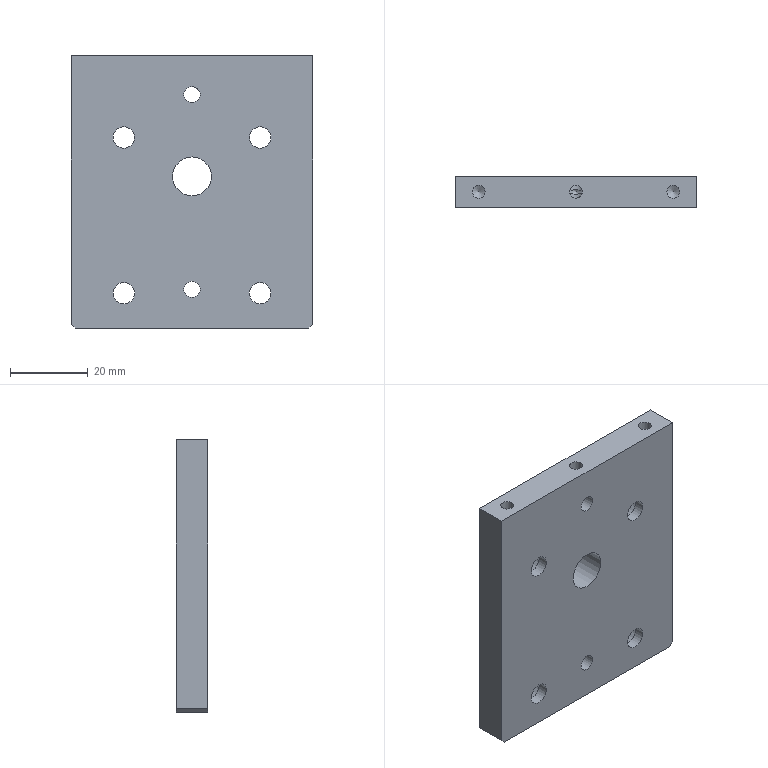Part | NX | 1 solid | 31 faces | box 62 x 8 x 70 mm | volume 31647 mm3 | cylinder 16 | plane 12 | cone 3 | commonest cylinder face diameters 3.3 x5 10 x5 5.5 x4 4.2 x2
STEP:
#1=CARTESIAN_POINT('',(-31.,4.,-34.));
#2=VERTEX_POINT('',#1);
#3=CARTESIAN_POINT('',(-31.,4.,35.));
#4=VERTEX_POINT('',#3);
#5=CARTESIAN_POINT('',(-31.,4.,35.));
#6=DIRECTION('',(0.,0.,1.));
#7=VECTOR('',#6,1000.);
#8=LINE('',#5,#7);
#9=EDGE_CURVE('',#2,#4,#8,.T.);
#10=ORIENTED_EDGE('',*,*,#9,.F.);
#11=CARTESIAN_POINT('',(-31.,-4.,-34.));
#12=VERTEX_POINT('',#11);
#13=CARTESIAN_POINT('',(-31.,4.,-34.));
#14=DIRECTION('',(0.,-1.,0.));
#15=VECTOR('',#14,1000.);
#16=LINE('',#13,#15);
#17=EDGE_CURVE('',#2,#12,#16,.T.);
#18=ORIENTED_EDGE('',*,*,#17,.T.);
#19=CARTESIAN_POINT('',(-31.,-4.,35.));
#20=VERTEX_POINT('',#19);
#21=CARTESIAN_POINT('',(-31.,-4.,35.));
#22=DIRECTION('',(0.,0.,1.));
#23=VECTOR('',#22,1000.);
#24=LINE('',#21,#23);
#25=EDGE_CURVE('',#12,#20,#24,.T.);
#26=ORIENTED_EDGE('',*,*,#25,.T.);
#27=CARTESIAN_POINT('',(-31.,4.,35.));
#28=DIRECTION('',(0.,-1.,0.));
#29=VECTOR('',#28,1000.);
#30=LINE('',#27,#29);
#31=EDGE_CURVE('',#4,#20,#30,.T.);
#32=ORIENTED_EDGE('',*,*,#31,.F.);
#33=EDGE_LOOP('',(#10,#18,#26,#32));
#34=FACE_BOUND('',#33,.T.);
#35=CARTESIAN_POINT('',(-31.,4.,35.));
#36=DIRECTION('',(1.,0.,0.));
#37=DIRECTION('',(0.,0.,-1.));
#38=AXIS2_PLACEMENT_3D('',#35,#36,#37);
#39=PLANE('',#38);
#40=ADVANCED_FACE('',(#34),#39,.F.);
#41=CARTESIAN_POINT('',(-23.35,0.,35.));
#42=VERTEX_POINT('',#41);
#43=CARTESIAN_POINT('',(-25.,0.,35.));
#44=DIRECTION('',(0.,0.,1.));
#45=DIRECTION('',(1.,0.,0.));
#46=AXIS2_PLACEMENT_3D('',#43,#44,#45);
#47=CIRCLE('',#46,1.65);
#48=EDGE_CURVE('',#42,#42,#47,.T.);
#49=ORIENTED_EDGE('',*,*,#48,.F.);
#50=EDGE_LOOP('',(#49));
#51=FACE_BOUND('',#50,.T.);
#52=CARTESIAN_POINT('',(1.65,0.,35.));
#53=VERTEX_POINT('',#52);
#54=CARTESIAN_POINT('',(0.,0.,35.));
#55=DIRECTION('',(0.,0.,1.));
#56=DIRECTION('',(1.,0.,0.));
#57=AXIS2_PLACEMENT_3D('',#54,#55,#56);
#58=CIRCLE('',#57,1.65);
#59=EDGE_CURVE('',#53,#53,#58,.T.);
#60=ORIENTED_EDGE('',*,*,#59,.F.);
#61=EDGE_LOOP('',(#60));
#62=FACE_BOUND('',#61,.T.);
#63=CARTESIAN_POINT('',(26.65,0.,35.));
#64=VERTEX_POINT('',#63);
#65=CARTESIAN_POINT('',(25.,0.,35.));
#66=DIRECTION('',(0.,0.,1.));
#67=DIRECTION('',(1.,0.,0.));
#68=AXIS2_PLACEMENT_3D('',#65,#66,#67);
#69=CIRCLE('',#68,1.65);
#70=EDGE_CURVE('',#64,#64,#69,.T.);
#71=ORIENTED_EDGE('',*,*,#70,.F.);
#72=EDGE_LOOP('',(#71));
#73=FACE_BOUND('',#72,.T.);
#74=CARTESIAN_POINT('',(31.,-4.,35.));
#75=VERTEX_POINT('',#74);
#76=CARTESIAN_POINT('',(31.,-4.,35.));
#77=DIRECTION('',(1.,0.,0.));
#78=VECTOR('',#77,1000.);
#79=LINE('',#76,#78);
#80=EDGE_CURVE('',#20,#75,#79,.T.);
#81=ORIENTED_EDGE('',*,*,#80,.T.);
#82=CARTESIAN_POINT('',(31.,4.,35.));
#83=VERTEX_POINT('',#82);
#84=CARTESIAN_POINT('',(31.,4.,35.));
#85=DIRECTION('',(0.,-1.,0.));
#86=VECTOR('',#85,1000.);
#87=LINE('',#84,#86);
#88=EDGE_CURVE('',#83,#75,#87,.T.);
#89=ORIENTED_EDGE('',*,*,#88,.F.);
#90=CARTESIAN_POINT('',(31.,4.,35.));
#91=DIRECTION('',(1.,0.,0.));
#92=VECTOR('',#91,1000.);
#93=LINE('',#90,#92);
#94=EDGE_CURVE('',#4,#83,#93,.T.);
#95=ORIENTED_EDGE('',*,*,#94,.F.);
#96=ORIENTED_EDGE('',*,*,#31,.T.);
#97=EDGE_LOOP('',(#81,#89,#95,#96));
#98=FACE_BOUND('',#97,.T.);
#99=CARTESIAN_POINT('',(31.,4.,35.));
#100=DIRECTION('',(0.,0.,-1.));
#101=DIRECTION('',(-1.,0.,0.));
#102=AXIS2_PLACEMENT_3D('',#99,#100,#101);
#103=PLANE('',#102);
#104=ADVANCED_FACE('',(#51,#62,#73,#98),#103,.F.);
#105=CARTESIAN_POINT('',(31.,-4.,-34.));
#106=VERTEX_POINT('',#105);
#107=CARTESIAN_POINT('',(31.,-4.,35.));
#108=DIRECTION('',(0.,0.,-1.));
#109=VECTOR('',#108,1000.);
#110=LINE('',#107,#109);
#111=EDGE_CURVE('',#75,#106,#110,.T.);
#112=ORIENTED_EDGE('',*,*,#111,.T.);
#113=CARTESIAN_POINT('',(31.,4.,-34.));
#114=VERTEX_POINT('',#113);
#115=CARTESIAN_POINT('',(31.,4.,-34.));
#116=DIRECTION('',(0.,1.,0.));
#117=VECTOR('',#116,1000.);
#118=LINE('',#115,#117);
#119=EDGE_CURVE('',#106,#114,#118,.T.);
#120=ORIENTED_EDGE('',*,*,#119,.T.);
#121=CARTESIAN_POINT('',(31.,4.,35.));
#122=DIRECTION('',(0.,0.,-1.));
#123=VECTOR('',#122,1000.);
#124=LINE('',#121,#123);
#125=EDGE_CURVE('',#83,#114,#124,.T.);
#126=ORIENTED_EDGE('',*,*,#125,.F.);
#127=ORIENTED_EDGE('',*,*,#88,.T.);
#128=EDGE_LOOP('',(#112,#120,#126,#127));
#129=FACE_BOUND('',#128,.T.);
#130=CARTESIAN_POINT('',(31.,4.,35.));
#131=DIRECTION('',(-1.,0.,0.));
#132=DIRECTION('',(0.,0.,1.));
#133=AXIS2_PLACEMENT_3D('',#130,#131,#132);
#134=PLANE('',#133);
#135=ADVANCED_FACE('',(#129),#134,.F.);
#136=CARTESIAN_POINT('',(30.,4.,-35.));
#137=VERTEX_POINT('',#136);
#138=CARTESIAN_POINT('',(-30.,4.,-35.));
#139=VERTEX_POINT('',#138);
#140=CARTESIAN_POINT('',(31.,4.,-35.));
#141=DIRECTION('',(-1.,0.,0.));
#142=VECTOR('',#141,1000.);
#143=LINE('',#140,#142);
#144=EDGE_CURVE('',#137,#139,#143,.T.);
#145=ORIENTED_EDGE('',*,*,#144,.F.);
#146=CARTESIAN_POINT('',(30.,-4.,-35.));
#147=VERTEX_POINT('',#146);
#148=CARTESIAN_POINT('',(30.,4.,-35.));
#149=DIRECTION('',(0.,-1.,0.));
#150=VECTOR('',#149,1000.);
#151=LINE('',#148,#150);
#152=EDGE_CURVE('',#137,#147,#151,.T.);
#153=ORIENTED_EDGE('',*,*,#152,.T.);
#154=CARTESIAN_POINT('',(-30.,-4.,-35.));
#155=VERTEX_POINT('',#154);
#156=CARTESIAN_POINT('',(31.,-4.,-35.));
#157=DIRECTION('',(-1.,0.,0.));
#158=VECTOR('',#157,1000.);
#159=LINE('',#156,#158);
#160=EDGE_CURVE('',#147,#155,#159,.T.);
#161=ORIENTED_EDGE('',*,*,#160,.T.);
#162=CARTESIAN_POINT('',(-30.,4.,-35.));
#163=DIRECTION('',(0.,1.,0.));
#164=VECTOR('',#163,1000.);
#165=LINE('',#162,#164);
#166=EDGE_CURVE('',#155,#139,#165,.T.);
#167=ORIENTED_EDGE('',*,*,#166,.T.);
#168=EDGE_LOOP('',(#145,#153,#161,#167));
#169=FACE_BOUND('',#168,.T.);
#170=CARTESIAN_POINT('',(31.,4.,-35.));
#171=DIRECTION('',(0.,0.,1.));
#172=DIRECTION('',(1.,0.,0.));
#173=AXIS2_PLACEMENT_3D('',#170,#171,#172);
#174=PLANE('',#173);
#175=ADVANCED_FACE('',(#169),#174,.F.);
#176=CARTESIAN_POINT('',(0.,4.,-22.9));
#177=VERTEX_POINT('',#176);
#178=CARTESIAN_POINT('',(0.,4.,-25.));
#179=DIRECTION('',(0.,1.,0.));
#180=DIRECTION('',(0.,0.,1.));
#181=AXIS2_PLACEMENT_3D('',#178,#179,#180);
#182=CIRCLE('',#181,2.1);
#183=EDGE_CURVE('',#177,#177,#182,.T.);
#184=ORIENTED_EDGE('',*,*,#183,.F.);
#185=EDGE_LOOP('',(#184));
#186=FACE_BOUND('',#185,.T.);
#187=CARTESIAN_POINT('',(0.,4.,27.1));
#188=VERTEX_POINT('',#187);
#189=CARTESIAN_POINT('',(0.,4.,25.));
#190=DIRECTION('',(0.,1.,0.));
#191=DIRECTION('',(0.,0.,1.));
#192=AXIS2_PLACEMENT_3D('',#189,#190,#191);
#193=CIRCLE('',#192,2.1);
#194=EDGE_CURVE('',#188,#188,#193,.T.);
#195=ORIENTED_EDGE('',*,*,#194,.F.);
#196=EDGE_LOOP('',(#195));
#197=FACE_BOUND('',#196,.T.);
#198=CARTESIAN_POINT('',(0.,4.,9.));
#199=VERTEX_POINT('',#198);
#200=CARTESIAN_POINT('',(0.,4.,4.));
#201=DIRECTION('',(0.,1.,0.));
#202=DIRECTION('',(0.,0.,1.));
#203=AXIS2_PLACEMENT_3D('',#200,#201,#202);
#204=CIRCLE('',#203,5.);
#205=EDGE_CURVE('',#199,#199,#204,.T.);
#206=ORIENTED_EDGE('',*,*,#205,.F.);
#207=EDGE_LOOP('',(#206));
#208=FACE_BOUND('',#207,.T.);
#209=CARTESIAN_POINT('',(-17.5,4.,-21.));
#210=VERTEX_POINT('',#209);
#211=CARTESIAN_POINT('',(-17.5,4.,-26.));
#212=DIRECTION('',(0.,1.,0.));
#213=DIRECTION('',(0.,0.,1.));
#214=AXIS2_PLACEMENT_3D('',#211,#212,#213);
#215=CIRCLE('',#214,5.);
#216=EDGE_CURVE('',#210,#210,#215,.T.);
#217=ORIENTED_EDGE('',*,*,#216,.F.);
#218=EDGE_LOOP('',(#217));
#219=FACE_BOUND('',#218,.T.);
#220=CARTESIAN_POINT('',(17.5,4.,-21.));
#221=VERTEX_POINT('',#220);
#222=CARTESIAN_POINT('',(17.5,4.,-26.));
#223=DIRECTION('',(0.,1.,0.));
#224=DIRECTION('',(0.,0.,1.));
#225=AXIS2_PLACEMENT_3D('',#222,#223,#224);
#226=CIRCLE('',#225,5.);
#227=EDGE_CURVE('',#221,#221,#226,.T.);
#228=ORIENTED_EDGE('',*,*,#227,.F.);
#229=EDGE_LOOP('',(#228));
#230=FACE_BOUND('',#229,.T.);
#231=CARTESIAN_POINT('',(-17.5,4.,19.));
#232=VERTEX_POINT('',#231);
#233=CARTESIAN_POINT('',(-17.5,4.,14.));
#234=DIRECTION('',(0.,1.,0.));
#235=DIRECTION('',(0.,0.,1.));
#236=AXIS2_PLACEMENT_3D('',#233,#234,#235);
#237=CIRCLE('',#236,5.);
#238=EDGE_CURVE('',#232,#232,#237,.T.);
#239=ORIENTED_EDGE('',*,*,#238,.F.);
#240=EDGE_LOOP('',(#239));
#241=FACE_BOUND('',#240,.T.);
#242=CARTESIAN_POINT('',(17.5,4.,19.));
#243=VERTEX_POINT('',#242);
#244=CARTESIAN_POINT('',(17.5,4.,14.));
#245=DIRECTION('',(0.,1.,0.));
#246=DIRECTION('',(0.,0.,1.));
#247=AXIS2_PLACEMENT_3D('',#244,#245,#246);
#248=CIRCLE('',#247,5.);
#249=EDGE_CURVE('',#243,#243,#248,.T.);
#250=ORIENTED_EDGE('',*,*,#249,.F.);
#251=EDGE_LOOP('',(#250));
#252=FACE_BOUND('',#251,.T.);
#253=ORIENTED_EDGE('',*,*,#125,.T.);
#254=CARTESIAN_POINT('',(32.5,4.,-32.5));
#255=DIRECTION('',(0.7071,0.,0.7071));
#256=VECTOR('',#255,1000.);
#257=LINE('',#254,#256);
#258=EDGE_CURVE('',#114,#137,#257,.F.);
#259=ORIENTED_EDGE('',*,*,#258,.T.);
#260=ORIENTED_EDGE('',*,*,#144,.T.);
#261=CARTESIAN_POINT('',(-32.5,4.,-32.5));
#262=DIRECTION('',(0.7071,0.,-0.7071));
#263=VECTOR('',#262,1000.);
#264=LINE('',#261,#263);
#265=EDGE_CURVE('',#139,#2,#264,.F.);
#266=ORIENTED_EDGE('',*,*,#265,.T.);
#267=ORIENTED_EDGE('',*,*,#9,.T.);
#268=ORIENTED_EDGE('',*,*,#94,.T.);
#269=EDGE_LOOP('',(#253,#259,#260,#266,#267,#268));
#270=FACE_BOUND('',#269,.T.);
#271=CARTESIAN_POINT('',(0.,4.,0.));
#272=DIRECTION('',(0.,1.,0.));
#273=DIRECTION('',(0.,0.,1.));
#274=AXIS2_PLACEMENT_3D('',#271,#272,#273);
#275=PLANE('',#274);
#276=ADVANCED_FACE('',(#186,#197,#208,#219,#230,#241,#252,#270),#275,.T.);
#277=CARTESIAN_POINT('',(0.,-4.,-22.9));
#278=VERTEX_POINT('',#277);
#279=CARTESIAN_POINT('',(0.,-4.,-25.));
#280=DIRECTION('',(0.,1.,0.));
#281=DIRECTION('',(0.,0.,1.));
#282=AXIS2_PLACEMENT_3D('',#279,#280,#281);
#283=CIRCLE('',#282,2.1);
#284=EDGE_CURVE('',#278,#278,#283,.T.);
#285=ORIENTED_EDGE('',*,*,#284,.T.);
#286=EDGE_LOOP('',(#285));
#287=FACE_BOUND('',#286,.T.);
#288=CARTESIAN_POINT('',(0.,-4.,27.1));
#289=VERTEX_POINT('',#288);
#290=CARTESIAN_POINT('',(0.,-4.,25.));
#291=DIRECTION('',(0.,1.,0.));
#292=DIRECTION('',(0.,0.,1.));
#293=AXIS2_PLACEMENT_3D('',#290,#291,#292);
#294=CIRCLE('',#293,2.1);
#295=EDGE_CURVE('',#289,#289,#294,.T.);
#296=ORIENTED_EDGE('',*,*,#295,.T.);
#297=EDGE_LOOP('',(#296));
#298=FACE_BOUND('',#297,.T.);
#299=CARTESIAN_POINT('',(0.,-4.,9.));
#300=VERTEX_POINT('',#299);
#301=CARTESIAN_POINT('',(0.,-4.,4.));
#302=DIRECTION('',(0.,1.,0.));
#303=DIRECTION('',(0.,0.,1.));
#304=AXIS2_PLACEMENT_3D('',#301,#302,#303);
#305=CIRCLE('',#304,5.);
#306=EDGE_CURVE('',#300,#300,#305,.T.);
#307=ORIENTED_EDGE('',*,*,#306,.T.);
#308=EDGE_LOOP('',(#307));
#309=FACE_BOUND('',#308,.T.);
#310=CARTESIAN_POINT('',(-17.5,-4.,-23.25));
#311=VERTEX_POINT('',#310);
#312=CARTESIAN_POINT('',(-17.5,-4.,-26.));
#313=DIRECTION('',(0.,1.,0.));
#314=DIRECTION('',(0.,0.,1.));
#315=AXIS2_PLACEMENT_3D('',#312,#313,#314);
#316=CIRCLE('',#315,2.75);
#317=EDGE_CURVE('',#311,#311,#316,.T.);
#318=ORIENTED_EDGE('',*,*,#317,.T.);
#319=EDGE_LOOP('',(#318));
#320=FACE_BOUND('',#319,.T.);
#321=CARTESIAN_POINT('',(17.5,-4.,-23.25));
#322=VERTEX_POINT('',#321);
#323=CARTESIAN_POINT('',(17.5,-4.,-26.));
#324=DIRECTION('',(0.,1.,0.));
#325=DIRECTION('',(0.,0.,1.));
#326=AXIS2_PLACEMENT_3D('',#323,#324,#325);
#327=CIRCLE('',#326,2.75);
#328=EDGE_CURVE('',#322,#322,#327,.T.);
#329=ORIENTED_EDGE('',*,*,#328,.T.);
#330=EDGE_LOOP('',(#329));
#331=FACE_BOUND('',#330,.T.);
#332=CARTESIAN_POINT('',(-17.5,-4.,16.75));
#333=VERTEX_POINT('',#332);
#334=CARTESIAN_POINT('',(-17.5,-4.,14.));
#335=DIRECTION('',(0.,1.,0.));
#336=DIRECTION('',(0.,0.,1.));
#337=AXIS2_PLACEMENT_3D('',#334,#335,#336);
#338=CIRCLE('',#337,2.75);
#339=EDGE_CURVE('',#333,#333,#338,.T.);
#340=ORIENTED_EDGE('',*,*,#339,.T.);
#341=EDGE_LOOP('',(#340));
#342=FACE_BOUND('',#341,.T.);
#343=CARTESIAN_POINT('',(17.5,-4.,16.75));
#344=VERTEX_POINT('',#343);
#345=CARTESIAN_POINT('',(17.5,-4.,14.));
#346=DIRECTION('',(0.,1.,0.));
#347=DIRECTION('',(0.,0.,1.));
#348=AXIS2_PLACEMENT_3D('',#345,#346,#347);
#349=CIRCLE('',#348,2.75);
#350=EDGE_CURVE('',#344,#344,#349,.T.);
#351=ORIENTED_EDGE('',*,*,#350,.T.);
#352=EDGE_LOOP('',(#351));
#353=FACE_BOUND('',#352,.T.);
#354=ORIENTED_EDGE('',*,*,#160,.F.);
#355=CARTESIAN_POINT('',(30.,-4.,-35.));
#356=DIRECTION('',(-0.7071,0.,-0.7071));
#357=VECTOR('',#356,1000.);
#358=LINE('',#355,#357);
#359=EDGE_CURVE('',#147,#106,#358,.F.);
#360=ORIENTED_EDGE('',*,*,#359,.T.);
#361=ORIENTED_EDGE('',*,*,#111,.F.);
#362=ORIENTED_EDGE('',*,*,#80,.F.);
#363=ORIENTED_EDGE('',*,*,#25,.F.);
#364=CARTESIAN_POINT('',(-31.,-4.,-34.));
#365=DIRECTION('',(-0.7071,0.,0.7071));
#366=VECTOR('',#365,1000.);
#367=LINE('',#364,#366);
#368=EDGE_CURVE('',#12,#155,#367,.F.);
#369=ORIENTED_EDGE('',*,*,#368,.T.);
#370=EDGE_LOOP('',(#354,#360,#361,#362,#363,#369));
#371=FACE_BOUND('',#370,.T.);
#372=CARTESIAN_POINT('',(0.,-4.,0.));
#373=DIRECTION('',(0.,1.,0.));
#374=DIRECTION('',(0.,0.,1.));
#375=AXIS2_PLACEMENT_3D('',#372,#373,#374);
#376=PLANE('',#375);
#377=ADVANCED_FACE('',(#287,#298,#309,#320,#331,#342,#353,#371),#376,.F.);
#378=ORIENTED_EDGE('',*,*,#350,.F.);
#379=EDGE_LOOP('',(#378));
#380=FACE_BOUND('',#379,.T.);
#381=CARTESIAN_POINT('',(17.5,-1.4,16.75));
#382=VERTEX_POINT('',#381);
#383=CARTESIAN_POINT('',(17.5,-1.4,14.));
#384=DIRECTION('',(0.,1.,0.));
#385=DIRECTION('',(0.,0.,1.));
#386=AXIS2_PLACEMENT_3D('',#383,#384,#385);
#387=CIRCLE('',#386,2.75);
#388=EDGE_CURVE('',#382,#382,#387,.T.);
#389=ORIENTED_EDGE('',*,*,#388,.T.);
#390=EDGE_LOOP('',(#389));
#391=FACE_BOUND('',#390,.T.);
#392=CARTESIAN_POINT('',(17.5,4.,14.));
#393=DIRECTION('',(0.,1.,0.));
#394=DIRECTION('',(0.,0.,1.));
#395=AXIS2_PLACEMENT_3D('',#392,#393,#394);
#396=CYLINDRICAL_SURFACE('',#395,2.75);
#397=ADVANCED_FACE('',(#380,#391),#396,.F.);
#398=ORIENTED_EDGE('',*,*,#388,.F.);
#399=EDGE_LOOP('',(#398));
#400=FACE_BOUND('',#399,.T.);
#401=CARTESIAN_POINT('',(17.5,-1.4,19.));
#402=VERTEX_POINT('',#401);
#403=CARTESIAN_POINT('',(17.5,-1.4,14.));
#404=DIRECTION('',(0.,1.,0.));
#405=DIRECTION('',(0.,0.,1.));
#406=AXIS2_PLACEMENT_3D('',#403,#404,#405);
#407=CIRCLE('',#406,5.);
#408=EDGE_CURVE('',#402,#402,#407,.T.);
#409=ORIENTED_EDGE('',*,*,#408,.T.);
#410=EDGE_LOOP('',(#409));
#411=FACE_BOUND('',#410,.T.);
#412=CARTESIAN_POINT('',(20.25,-1.4,14.));
#413=DIRECTION('',(0.,-1.,0.));
#414=DIRECTION('',(0.,0.,-1.));
#415=AXIS2_PLACEMENT_3D('',#412,#413,#414);
#416=PLANE('',#415);
#417=ADVANCED_FACE('',(#400,#411),#416,.F.);
#418=ORIENTED_EDGE('',*,*,#408,.F.);
#419=EDGE_LOOP('',(#418));
#420=FACE_BOUND('',#419,.T.);
#421=ORIENTED_EDGE('',*,*,#249,.T.);
#422=EDGE_LOOP('',(#421));
#423=FACE_BOUND('',#422,.T.);
#424=CARTESIAN_POINT('',(17.5,4.,14.));
#425=DIRECTION('',(0.,1.,0.));
#426=DIRECTION('',(0.,0.,1.));
#427=AXIS2_PLACEMENT_3D('',#424,#425,#426);
#428=CYLINDRICAL_SURFACE('',#427,5.);
#429=ADVANCED_FACE('',(#420,#423),#428,.F.);
#430=ORIENTED_EDGE('',*,*,#339,.F.);
#431=EDGE_LOOP('',(#430));
#432=FACE_BOUND('',#431,.T.);
#433=CARTESIAN_POINT('',(-17.5,-1.4,16.75));
#434=VERTEX_POINT('',#433);
#435=CARTESIAN_POINT('',(-17.5,-1.4,14.));
#436=DIRECTION('',(0.,1.,0.));
#437=DIRECTION('',(0.,0.,1.));
#438=AXIS2_PLACEMENT_3D('',#435,#436,#437);
#439=CIRCLE('',#438,2.75);
#440=EDGE_CURVE('',#434,#434,#439,.T.);
#441=ORIENTED_EDGE('',*,*,#440,.T.);
#442=EDGE_LOOP('',(#441));
#443=FACE_BOUND('',#442,.T.);
#444=CARTESIAN_POINT('',(-17.5,4.,14.));
#445=DIRECTION('',(0.,1.,0.));
#446=DIRECTION('',(0.,0.,1.));
#447=AXIS2_PLACEMENT_3D('',#444,#445,#446);
#448=CYLINDRICAL_SURFACE('',#447,2.75);
#449=ADVANCED_FACE('',(#432,#443),#448,.F.);
#450=ORIENTED_EDGE('',*,*,#440,.F.);
#451=EDGE_LOOP('',(#450));
#452=FACE_BOUND('',#451,.T.);
#453=CARTESIAN_POINT('',(-17.5,-1.4,19.));
#454=VERTEX_POINT('',#453);
#455=CARTESIAN_POINT('',(-17.5,-1.4,14.));
#456=DIRECTION('',(0.,1.,0.));
#457=DIRECTION('',(0.,0.,1.));
#458=AXIS2_PLACEMENT_3D('',#455,#456,#457);
#459=CIRCLE('',#458,5.);
#460=EDGE_CURVE('',#454,#454,#459,.T.);
#461=ORIENTED_EDGE('',*,*,#460,.T.);
#462=EDGE_LOOP('',(#461));
#463=FACE_BOUND('',#462,.T.);
#464=CARTESIAN_POINT('',(-14.75,-1.4,14.));
#465=DIRECTION('',(0.,-1.,0.));
#466=DIRECTION('',(0.,0.,-1.));
#467=AXIS2_PLACEMENT_3D('',#464,#465,#466);
#468=PLANE('',#467);
#469=ADVANCED_FACE('',(#452,#463),#468,.F.);
#470=ORIENTED_EDGE('',*,*,#460,.F.);
#471=EDGE_LOOP('',(#470));
#472=FACE_BOUND('',#471,.T.);
#473=ORIENTED_EDGE('',*,*,#238,.T.);
#474=EDGE_LOOP('',(#473));
#475=FACE_BOUND('',#474,.T.);
#476=CARTESIAN_POINT('',(-17.5,4.,14.));
#477=DIRECTION('',(0.,1.,0.));
#478=DIRECTION('',(0.,0.,1.));
#479=AXIS2_PLACEMENT_3D('',#476,#477,#478);
#480=CYLINDRICAL_SURFACE('',#479,5.);
#481=ADVANCED_FACE('',(#472,#475),#480,.F.);
#482=ORIENTED_EDGE('',*,*,#328,.F.);
#483=EDGE_LOOP('',(#482));
#484=FACE_BOUND('',#483,.T.);
#485=CARTESIAN_POINT('',(17.5,-1.4,-23.25));
#486=VERTEX_POINT('',#485);
#487=CARTESIAN_POINT('',(17.5,-1.4,-26.));
#488=DIRECTION('',(0.,1.,0.));
#489=DIRECTION('',(0.,0.,1.));
#490=AXIS2_PLACEMENT_3D('',#487,#488,#489);
#491=CIRCLE('',#490,2.75);
#492=EDGE_CURVE('',#486,#486,#491,.T.);
#493=ORIENTED_EDGE('',*,*,#492,.T.);
#494=EDGE_LOOP('',(#493));
#495=FACE_BOUND('',#494,.T.);
#496=CARTESIAN_POINT('',(17.5,4.,-26.));
#497=DIRECTION('',(0.,1.,0.));
#498=DIRECTION('',(0.,0.,1.));
#499=AXIS2_PLACEMENT_3D('',#496,#497,#498);
#500=CYLINDRICAL_SURFACE('',#499,2.75);
#501=ADVANCED_FACE('',(#484,#495),#500,.F.);
#502=ORIENTED_EDGE('',*,*,#492,.F.);
#503=EDGE_LOOP('',(#502));
#504=FACE_BOUND('',#503,.T.);
#505=CARTESIAN_POINT('',(17.5,-1.4,-21.));
#506=VERTEX_POINT('',#505);
#507=CARTESIAN_POINT('',(17.5,-1.4,-26.));
#508=DIRECTION('',(0.,1.,0.));
#509=DIRECTION('',(0.,0.,1.));
#510=AXIS2_PLACEMENT_3D('',#507,#508,#509);
#511=CIRCLE('',#510,5.);
#512=EDGE_CURVE('',#506,#506,#511,.T.);
#513=ORIENTED_EDGE('',*,*,#512,.T.);
#514=EDGE_LOOP('',(#513));
#515=FACE_BOUND('',#514,.T.);
#516=CARTESIAN_POINT('',(20.25,-1.4,-26.));
#517=DIRECTION('',(0.,-1.,0.));
#518=DIRECTION('',(0.,0.,-1.));
#519=AXIS2_PLACEMENT_3D('',#516,#517,#518);
#520=PLANE('',#519);
#521=ADVANCED_FACE('',(#504,#515),#520,.F.);
#522=ORIENTED_EDGE('',*,*,#512,.F.);
#523=EDGE_LOOP('',(#522));
#524=FACE_BOUND('',#523,.T.);
#525=ORIENTED_EDGE('',*,*,#227,.T.);
#526=EDGE_LOOP('',(#525));
#527=FACE_BOUND('',#526,.T.);
#528=CARTESIAN_POINT('',(17.5,4.,-26.));
#529=DIRECTION('',(0.,1.,0.));
#530=DIRECTION('',(0.,0.,1.));
#531=AXIS2_PLACEMENT_3D('',#528,#529,#530);
#532=CYLINDRICAL_SURFACE('',#531,5.);
#533=ADVANCED_FACE('',(#524,#527),#532,.F.);
#534=ORIENTED_EDGE('',*,*,#317,.F.);
#535=EDGE_LOOP('',(#534));
#536=FACE_BOUND('',#535,.T.);
#537=CARTESIAN_POINT('',(-17.5,-1.4,-23.25));
#538=VERTEX_POINT('',#537);
#539=CARTESIAN_POINT('',(-17.5,-1.4,-26.));
#540=DIRECTION('',(0.,1.,0.));
#541=DIRECTION('',(0.,0.,1.));
#542=AXIS2_PLACEMENT_3D('',#539,#540,#541);
#543=CIRCLE('',#542,2.75);
#544=EDGE_CURVE('',#538,#538,#543,.T.);
#545=ORIENTED_EDGE('',*,*,#544,.T.);
#546=EDGE_LOOP('',(#545));
#547=FACE_BOUND('',#546,.T.);
#548=CARTESIAN_POINT('',(-17.5,4.,-26.));
#549=DIRECTION('',(0.,1.,0.));
#550=DIRECTION('',(0.,0.,1.));
#551=AXIS2_PLACEMENT_3D('',#548,#549,#550);
#552=CYLINDRICAL_SURFACE('',#551,2.75);
#553=ADVANCED_FACE('',(#536,#547),#552,.F.);
#554=ORIENTED_EDGE('',*,*,#544,.F.);
#555=EDGE_LOOP('',(#554));
#556=FACE_BOUND('',#555,.T.);
#557=CARTESIAN_POINT('',(-17.5,-1.4,-21.));
#558=VERTEX_POINT('',#557);
#559=CARTESIAN_POINT('',(-17.5,-1.4,-26.));
#560=DIRECTION('',(0.,1.,0.));
#561=DIRECTION('',(0.,0.,1.));
#562=AXIS2_PLACEMENT_3D('',#559,#560,#561);
#563=CIRCLE('',#562,5.);
#564=EDGE_CURVE('',#558,#558,#563,.T.);
#565=ORIENTED_EDGE('',*,*,#564,.T.);
#566=EDGE_LOOP('',(#565));
#567=FACE_BOUND('',#566,.T.);
#568=CARTESIAN_POINT('',(-14.75,-1.4,-26.));
#569=DIRECTION('',(0.,-1.,0.));
#570=DIRECTION('',(0.,0.,-1.));
#571=AXIS2_PLACEMENT_3D('',#568,#569,#570);
#572=PLANE('',#571);
#573=ADVANCED_FACE('',(#556,#567),#572,.F.);
#574=ORIENTED_EDGE('',*,*,#564,.F.);
#575=EDGE_LOOP('',(#574));
#576=FACE_BOUND('',#575,.T.);
#577=ORIENTED_EDGE('',*,*,#216,.T.);
#578=EDGE_LOOP('',(#577));
#579=FACE_BOUND('',#578,.T.);
#580=CARTESIAN_POINT('',(-17.5,4.,-26.));
#581=DIRECTION('',(0.,1.,0.));
#582=DIRECTION('',(0.,0.,1.));
#583=AXIS2_PLACEMENT_3D('',#580,#581,#582);
#584=CYLINDRICAL_SURFACE('',#583,5.);
#585=ADVANCED_FACE('',(#576,#579),#584,.F.);
#586=CARTESIAN_POINT('',(25.,0.,22.509));
#587=VERTEX_POINT('',#586);
#588=VERTEX_LOOP('',#587);
#589=FACE_BOUND('',#588,.T.);
#590=CARTESIAN_POINT('',(26.65,0.,23.5));
#591=VERTEX_POINT('',#590);
#592=CARTESIAN_POINT('',(25.,0.,23.5));
#593=DIRECTION('',(0.,0.,1.));
#594=DIRECTION('',(1.,0.,0.));
#595=AXIS2_PLACEMENT_3D('',#592,#593,#594);
#596=CIRCLE('',#595,1.65);
#597=EDGE_CURVE('',#591,#591,#596,.T.);
#598=ORIENTED_EDGE('',*,*,#597,.T.);
#599=EDGE_LOOP('',(#598));
#600=FACE_BOUND('',#599,.T.);
#601=CARTESIAN_POINT('',(25.,0.,23.5));
#602=DIRECTION('',(0.,0.,1.));
#603=DIRECTION('',(1.,0.,0.));
#604=AXIS2_PLACEMENT_3D('',#601,#602,#603);
#605=CONICAL_SURFACE('',#604,1.65,1.03);
#606=ADVANCED_FACE('',(#589,#600),#605,.F.);
#607=ORIENTED_EDGE('',*,*,#597,.F.);
#608=EDGE_LOOP('',(#607));
#609=FACE_BOUND('',#608,.T.);
#610=ORIENTED_EDGE('',*,*,#70,.T.);
#611=EDGE_LOOP('',(#610));
#612=FACE_BOUND('',#611,.T.);
#613=CARTESIAN_POINT('',(25.,0.,35.));
#614=DIRECTION('',(0.,0.,1.));
#615=DIRECTION('',(1.,0.,0.));
#616=AXIS2_PLACEMENT_3D('',#613,#614,#615);
#617=CYLINDRICAL_SURFACE('',#616,1.65);
#618=ADVANCED_FACE('',(#609,#612),#617,.F.);
#619=CARTESIAN_POINT('',(1.65,0.,26.299));
#620=VERTEX_POINT('',#619);
#621=CARTESIAN_POINT('',(1.55,0.6771,26.43));
#622=CARTESIAN_POINT('',(1.744,-0.2353,26.172));
#623=CARTESIAN_POINT('',(1.307,-1.268,26.781));
#624=CARTESIAN_POINT('',(0.004688,-1.838,27.259));
#625=CARTESIAN_POINT('',(-1.307,-1.279,26.782));
#626=CARTESIAN_POINT('',(-1.821,-0.0003141,26.059));
#627=CARTESIAN_POINT('',(-1.309,1.273,26.778));
#628=CARTESIAN_POINT('',(-0.007469,1.844,27.262));
#629=CARTESIAN_POINT('',(1.097,1.351,26.856));
#630=CARTESIAN_POINT('',(1.55,0.6771,26.43));
#631=CARTESIAN_POINT('',(1.744,-0.2353,26.172));
#632=CARTESIAN_POINT('',(1.307,-1.268,26.781));
#633=B_SPLINE_CURVE_WITH_KNOTS('',3,(#621,#622,#623,#624,#625,#626,#627,#628,#629,#630,#631,#632),.UNSPECIFIED.,.T.,.F.,(1,1,1,1,1,1,1,1,1,1,1,1,1,1,1,1),(-0.002727,-0.001364,-0.0006818,0.,0.001364,0.002727,0.004091,0.005454,0.006818,0.008181,0.009545,0.01023,0.01091,0.01227,0.01364,0.015),.UNSPECIFIED.);
#634=EDGE_CURVE('',#620,#620,#633,.T.);
#635=ORIENTED_EDGE('',*,*,#634,.T.);
#636=EDGE_LOOP('',(#635));
#637=FACE_BOUND('',#636,.T.);
#638=ORIENTED_EDGE('',*,*,#59,.T.);
#639=EDGE_LOOP('',(#638));
#640=FACE_BOUND('',#639,.T.);
#641=CARTESIAN_POINT('',(0.,0.,35.));
#642=DIRECTION('',(0.,0.,1.));
#643=DIRECTION('',(1.,0.,0.));
#644=AXIS2_PLACEMENT_3D('',#641,#642,#643);
#645=CYLINDRICAL_SURFACE('',#644,1.65);
#646=ADVANCED_FACE('',(#637,#640),#645,.F.);
#647=CARTESIAN_POINT('',(-25.,0.,22.509));
#648=VERTEX_POINT('',#647);
#649=VERTEX_LOOP('',#648);
#650=FACE_BOUND('',#649,.T.);
#651=CARTESIAN_POINT('',(-23.35,0.,23.5));
#652=VERTEX_POINT('',#651);
#653=CARTESIAN_POINT('',(-25.,0.,23.5));
#654=DIRECTION('',(0.,0.,1.));
#655=DIRECTION('',(1.,0.,0.));
#656=AXIS2_PLACEMENT_3D('',#653,#654,#655);
#657=CIRCLE('',#656,1.65);
#658=EDGE_CURVE('',#652,#652,#657,.T.);
#659=ORIENTED_EDGE('',*,*,#658,.T.);
#660=EDGE_LOOP('',(#659));
#661=FACE_BOUND('',#660,.T.);
#662=CARTESIAN_POINT('',(-25.,0.,23.5));
#663=DIRECTION('',(0.,0.,1.));
#664=DIRECTION('',(1.,0.,0.));
#665=AXIS2_PLACEMENT_3D('',#662,#663,#664);
#666=CONICAL_SURFACE('',#665,1.65,1.03);
#667=ADVANCED_FACE('',(#650,#661),#666,.F.);
#668=ORIENTED_EDGE('',*,*,#658,.F.);
#669=EDGE_LOOP('',(#668));
#670=FACE_BOUND('',#669,.T.);
#671=ORIENTED_EDGE('',*,*,#48,.T.);
#672=EDGE_LOOP('',(#671));
#673=FACE_BOUND('',#672,.T.);
#674=CARTESIAN_POINT('',(-25.,0.,35.));
#675=DIRECTION('',(0.,0.,1.));
#676=DIRECTION('',(1.,0.,0.));
#677=AXIS2_PLACEMENT_3D('',#674,#675,#676);
#678=CYLINDRICAL_SURFACE('',#677,1.65);
#679=ADVANCED_FACE('',(#670,#673),#678,.F.);
#680=ORIENTED_EDGE('',*,*,#306,.F.);
#681=EDGE_LOOP('',(#680));
#682=FACE_BOUND('',#681,.T.);
#683=ORIENTED_EDGE('',*,*,#205,.T.);
#684=EDGE_LOOP('',(#683));
#685=FACE_BOUND('',#684,.T.);
#686=CARTESIAN_POINT('',(0.,4.,4.));
#687=DIRECTION('',(0.,1.,0.));
#688=DIRECTION('',(0.,0.,1.));
#689=AXIS2_PLACEMENT_3D('',#686,#687,#688);
#690=CYLINDRICAL_SURFACE('',#689,5.);
#691=ADVANCED_FACE('',(#682,#685),#690,.F.);
#692=CARTESIAN_POINT('',(1.47,-0.75,23.5));
#693=VERTEX_POINT('',#692);
#694=CARTESIAN_POINT('',(1.47,0.75,23.5));
#695=VERTEX_POINT('',#694);
#696=CARTESIAN_POINT('',(1.47,-0.75,23.5));
#697=CARTESIAN_POINT('',(1.582,-0.5289,23.611));
#698=CARTESIAN_POINT('',(1.718,0.0006377,23.791));
#699=CARTESIAN_POINT('',(1.582,0.529,23.61));
#700=CARTESIAN_POINT('',(1.47,0.75,23.5));
#701=B_SPLINE_CURVE_WITH_KNOTS('',3,(#696,#697,#698,#699,#700),.UNSPECIFIED.,.F.,.F.,(4,1,4),(0.,0.000808,0.001616),.UNSPECIFIED.);
#702=EDGE_CURVE('',#693,#695,#701,.T.);
#703=ORIENTED_EDGE('',*,*,#702,.F.);
#704=CARTESIAN_POINT('',(-1.47,-0.75,23.5));
#705=VERTEX_POINT('',#704);
#706=CARTESIAN_POINT('',(-1.47,-0.75,23.5));
#707=CARTESIAN_POINT('',(-1.4,-0.6365,23.432));
#708=CARTESIAN_POINT('',(-1.245,-0.3853,23.291));
#709=CARTESIAN_POINT('',(-0.8317,-0.3978,23.054));
#710=CARTESIAN_POINT('',(-0.4462,-0.6058,22.934));
#711=CARTESIAN_POINT('',(0.002215,-0.6746,22.883));
#712=CARTESIAN_POINT('',(0.4495,-0.6046,22.935));
#713=CARTESIAN_POINT('',(0.8354,-0.3961,23.056));
#714=CARTESIAN_POINT('',(1.245,-0.3866,23.292));
#715=CARTESIAN_POINT('',(1.4,-0.6366,23.432));
#716=CARTESIAN_POINT('',(1.47,-0.75,23.5));
#717=B_SPLINE_CURVE_WITH_KNOTS('',3,(#706,#707,#708,#709,#710,#711,#712,#713,#714,#715,#716),.UNSPECIFIED.,.F.,.F.,(4,1,1,1,1,1,1,1,4),(0.0001321,0.0005805,0.001029,0.001477,0.001926,0.002374,0.002823,0.003271,0.00372),.UNSPECIFIED.);
#718=EDGE_CURVE('',#705,#693,#717,.T.);
#719=ORIENTED_EDGE('',*,*,#718,.F.);
#720=CARTESIAN_POINT('',(-1.47,0.75,23.5));
#721=VERTEX_POINT('',#720);
#722=CARTESIAN_POINT('',(-1.47,0.75,23.5));
#723=CARTESIAN_POINT('',(-1.582,0.5289,23.611));
#724=CARTESIAN_POINT('',(-1.718,-0.0006377,23.791));
#725=CARTESIAN_POINT('',(-1.582,-0.529,23.61));
#726=CARTESIAN_POINT('',(-1.47,-0.75,23.5));
#727=B_SPLINE_CURVE_WITH_KNOTS('',3,(#722,#723,#724,#725,#726),.UNSPECIFIED.,.F.,.F.,(4,1,4),(0.,0.000808,0.001616),.UNSPECIFIED.);
#728=EDGE_CURVE('',#721,#705,#727,.T.);
#729=ORIENTED_EDGE('',*,*,#728,.F.);
#730=CARTESIAN_POINT('',(1.47,0.75,23.5));
#731=CARTESIAN_POINT('',(1.4,0.6365,23.432));
#732=CARTESIAN_POINT('',(1.245,0.3853,23.291));
#733=CARTESIAN_POINT('',(0.8317,0.3978,23.054));
#734=CARTESIAN_POINT('',(0.4462,0.6058,22.934));
#735=CARTESIAN_POINT('',(-0.002215,0.6746,22.883));
#736=CARTESIAN_POINT('',(-0.4495,0.6046,22.935));
#737=CARTESIAN_POINT('',(-0.8354,0.3961,23.056));
#738=CARTESIAN_POINT('',(-1.245,0.3866,23.292));
#739=CARTESIAN_POINT('',(-1.4,0.6366,23.432));
#740=CARTESIAN_POINT('',(-1.47,0.75,23.5));
#741=B_SPLINE_CURVE_WITH_KNOTS('',3,(#730,#731,#732,#733,#734,#735,#736,#737,#738,#739,#740),.UNSPECIFIED.,.F.,.F.,(4,1,1,1,1,1,1,1,4),(0.0001321,0.0005805,0.001029,0.001477,0.001926,0.002374,0.002823,0.003271,0.00372),.UNSPECIFIED.);
#742=EDGE_CURVE('',#695,#721,#741,.T.);
#743=ORIENTED_EDGE('',*,*,#742,.F.);
#744=EDGE_LOOP('',(#703,#719,#729,#743));
#745=FACE_BOUND('',#744,.T.);
#746=ORIENTED_EDGE('',*,*,#295,.F.);
#747=EDGE_LOOP('',(#746));
#748=FACE_BOUND('',#747,.T.);
#749=ORIENTED_EDGE('',*,*,#194,.T.);
#750=EDGE_LOOP('',(#749));
#751=FACE_BOUND('',#750,.T.);
#752=ORIENTED_EDGE('',*,*,#634,.F.);
#753=EDGE_LOOP('',(#752));
#754=FACE_BOUND('',#753,.T.);
#755=CARTESIAN_POINT('',(0.,4.,25.));
#756=DIRECTION('',(0.,1.,0.));
#757=DIRECTION('',(0.,0.,1.));
#758=AXIS2_PLACEMENT_3D('',#755,#756,#757);
#759=CYLINDRICAL_SURFACE('',#758,2.1);
#760=ADVANCED_FACE('',(#745,#748,#751,#754),#759,.F.);
#761=CARTESIAN_POINT('',(0.,0.,22.509));
#762=VERTEX_POINT('',#761);
#763=VERTEX_LOOP('',#762);
#764=FACE_BOUND('',#763,.T.);
#765=CARTESIAN_POINT('',(0.,0.,23.5));
#766=DIRECTION('',(0.,0.,1.));
#767=DIRECTION('',(1.,0.,0.));
#768=AXIS2_PLACEMENT_3D('',#765,#766,#767);
#769=CIRCLE('',#768,1.65);
#770=EDGE_CURVE('',#693,#695,#769,.T.);
#771=ORIENTED_EDGE('',*,*,#770,.T.);
#772=ORIENTED_EDGE('',*,*,#742,.T.);
#773=CARTESIAN_POINT('',(0.,0.,23.5));
#774=DIRECTION('',(0.,0.,1.));
#775=DIRECTION('',(1.,0.,0.));
#776=AXIS2_PLACEMENT_3D('',#773,#774,#775);
#777=CIRCLE('',#776,1.65);
#778=EDGE_CURVE('',#721,#705,#777,.T.);
#779=ORIENTED_EDGE('',*,*,#778,.T.);
#780=ORIENTED_EDGE('',*,*,#718,.T.);
#781=EDGE_LOOP('',(#771,#772,#779,#780));
#782=FACE_BOUND('',#781,.T.);
#783=CARTESIAN_POINT('',(0.,0.,23.5));
#784=DIRECTION('',(0.,0.,1.));
#785=DIRECTION('',(1.,0.,0.));
#786=AXIS2_PLACEMENT_3D('',#783,#784,#785);
#787=CONICAL_SURFACE('',#786,1.65,1.03);
#788=ADVANCED_FACE('',(#764,#782),#787,.F.);
#789=ORIENTED_EDGE('',*,*,#778,.F.);
#790=ORIENTED_EDGE('',*,*,#728,.T.);
#791=EDGE_LOOP('',(#789,#790));
#792=FACE_BOUND('',#791,.T.);
#793=CARTESIAN_POINT('',(0.,0.,35.));
#794=DIRECTION('',(0.,0.,1.));
#795=DIRECTION('',(1.,0.,0.));
#796=AXIS2_PLACEMENT_3D('',#793,#794,#795);
#797=CYLINDRICAL_SURFACE('',#796,1.65);
#798=ADVANCED_FACE('',(#792),#797,.F.);
#799=ORIENTED_EDGE('',*,*,#770,.F.);
#800=ORIENTED_EDGE('',*,*,#702,.T.);
#801=EDGE_LOOP('',(#799,#800));
#802=FACE_BOUND('',#801,.T.);
#803=CARTESIAN_POINT('',(0.,0.,35.));
#804=DIRECTION('',(0.,0.,1.));
#805=DIRECTION('',(1.,0.,0.));
#806=AXIS2_PLACEMENT_3D('',#803,#804,#805);
#807=CYLINDRICAL_SURFACE('',#806,1.65);
#808=ADVANCED_FACE('',(#802),#807,.F.);
#809=ORIENTED_EDGE('',*,*,#284,.F.);
#810=EDGE_LOOP('',(#809));
#811=FACE_BOUND('',#810,.T.);
#812=ORIENTED_EDGE('',*,*,#183,.T.);
#813=EDGE_LOOP('',(#812));
#814=FACE_BOUND('',#813,.T.);
#815=CARTESIAN_POINT('',(0.,4.,-25.));
#816=DIRECTION('',(0.,1.,0.));
#817=DIRECTION('',(0.,0.,1.));
#818=AXIS2_PLACEMENT_3D('',#815,#816,#817);
#819=CYLINDRICAL_SURFACE('',#818,2.1);
#820=ADVANCED_FACE('',(#811,#814),#819,.F.);
#821=ORIENTED_EDGE('',*,*,#258,.F.);
#822=ORIENTED_EDGE('',*,*,#119,.F.);
#823=ORIENTED_EDGE('',*,*,#359,.F.);
#824=ORIENTED_EDGE('',*,*,#152,.F.);
#825=EDGE_LOOP('',(#821,#822,#823,#824));
#826=FACE_BOUND('',#825,.T.);
#827=CARTESIAN_POINT('',(30.,4.,-35.));
#828=DIRECTION('',(-0.7071,0.,0.7071));
#829=DIRECTION('',(0.,-1.,0.));
#830=AXIS2_PLACEMENT_3D('',#827,#828,#829);
#831=PLANE('',#830);
#832=ADVANCED_FACE('',(#826),#831,.F.);
#833=ORIENTED_EDGE('',*,*,#265,.F.);
#834=ORIENTED_EDGE('',*,*,#166,.F.);
#835=ORIENTED_EDGE('',*,*,#368,.F.);
#836=ORIENTED_EDGE('',*,*,#17,.F.);
#837=EDGE_LOOP('',(#833,#834,#835,#836));
#838=FACE_BOUND('',#837,.T.);
#839=CARTESIAN_POINT('',(-31.,4.,-34.));
#840=DIRECTION('',(0.7071,0.,0.7071));
#841=DIRECTION('',(0.,-1.,0.));
#842=AXIS2_PLACEMENT_3D('',#839,#840,#841);
#843=PLANE('',#842);
#844=ADVANCED_FACE('',(#838),#843,.F.);
#845=CLOSED_SHELL('',(#40,#104,#135,#175,#276,#377,#397,#417,#429,#449,#469,#481,#501,#521,#533,#553,#573,#585,#606,#618,#646,#667,#679,#691,#760,#788,#798,#808,#820,#832,#844));
#846=MANIFOLD_SOLID_BREP('',#845);
#847=(LENGTH_UNIT()NAMED_UNIT(*)SI_UNIT(.MILLI.,.METRE.));
#848=UNCERTAINTY_MEASURE_WITH_UNIT(LENGTH_MEASURE(0.0508),#847,'','');
#849=(NAMED_UNIT(*)PLANE_ANGLE_UNIT()SI_UNIT($,.RADIAN.));
#850=(NAMED_UNIT(*)SI_UNIT($,.STERADIAN.)SOLID_ANGLE_UNIT());
#851=(GEOMETRIC_REPRESENTATION_CONTEXT(3)GLOBAL_UNCERTAINTY_ASSIGNED_CONTEXT((#848))GLOBAL_UNIT_ASSIGNED_CONTEXT((#847,#849,#850))REPRESENTATION_CONTEXT('',''));
#852=ADVANCED_BREP_SHAPE_REPRESENTATION('',(#846),#851);